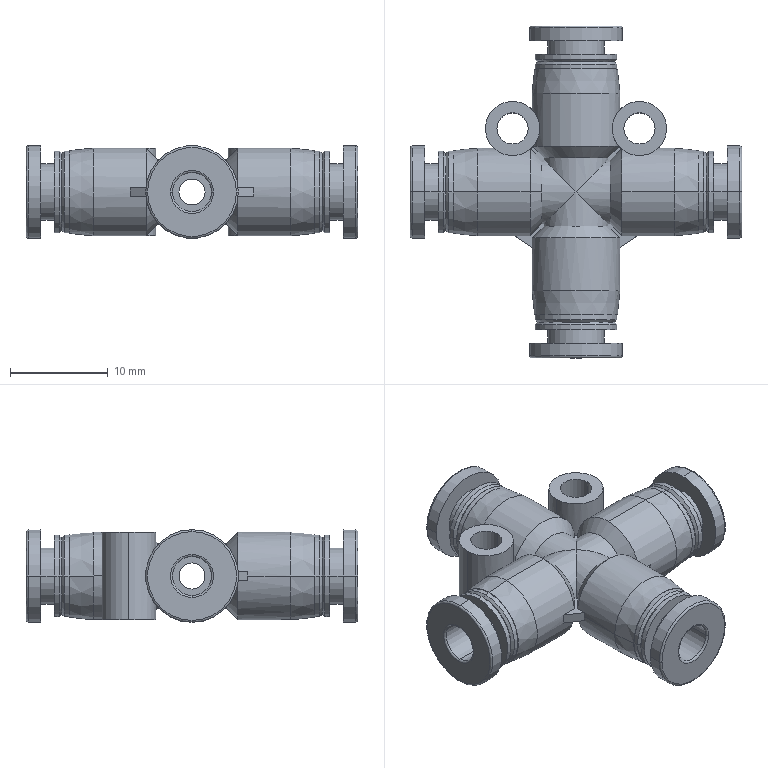Part | STEP file | Tube fitting PZ4 | 1 solid | 158 faces | box 34 x 34 x 9.5 mm | volume 2906 mm3 | cylinder 74 | cone 34 | plane 34 | torus 16 | commonest cylinder face diameters 8.4 x16 6.6 x10 2.667 x8 4 x8 5.8 x8 9 x8